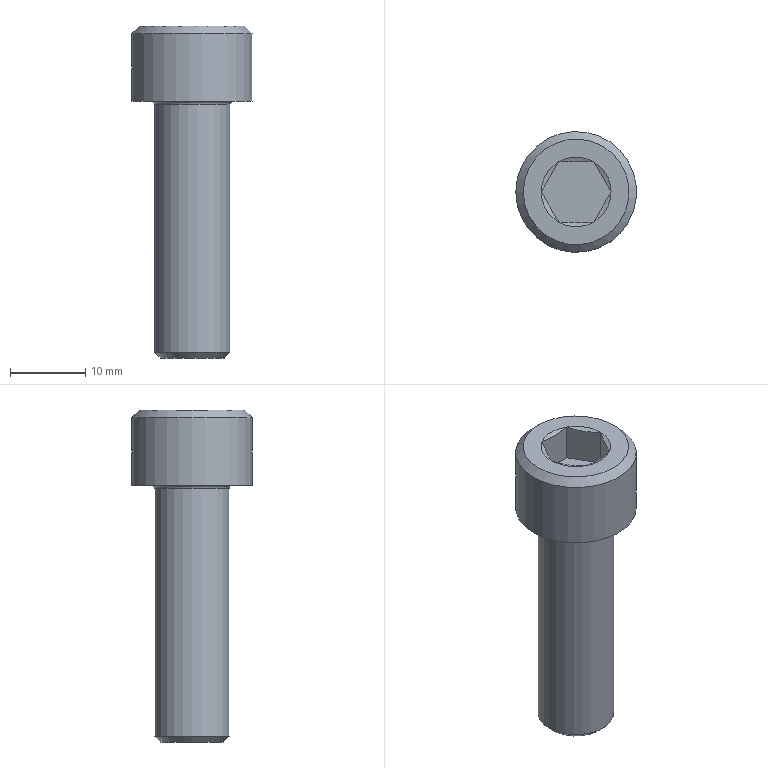Part | STEP file | solid 77 | 1 solid | 21 faces | box 16 x 16 x 44 mm | volume 4371 mm3 | plane 10 | sphere 6 | cylinder 2 | cone 2 | torus 1 | commonest cylinder face diameters 10 x1 16 x1